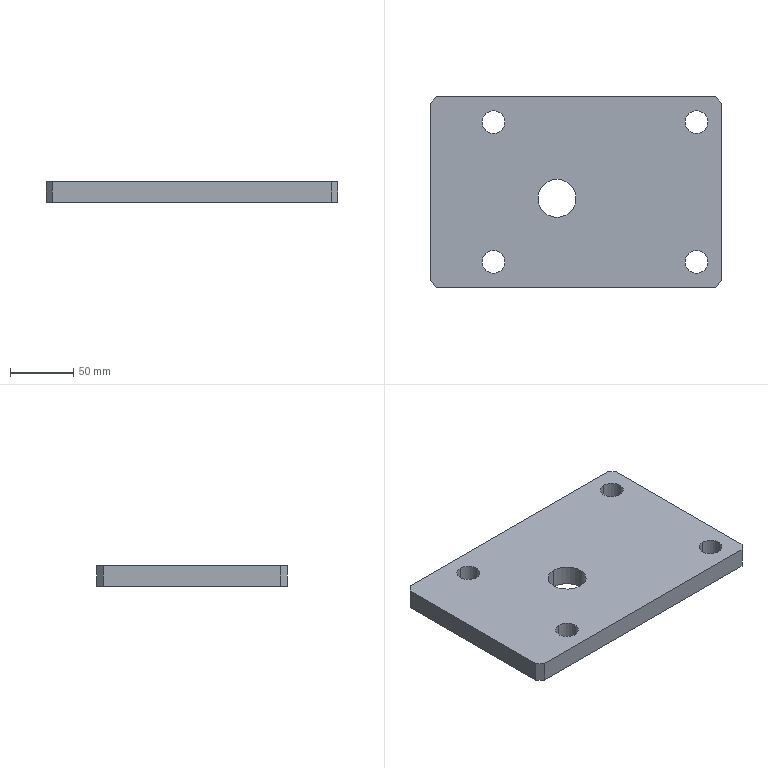Part | STEP file | [02]-1 | 1 solid | 20 faces | box 230 x 150 x 16 mm | volume 523604 mm3 | cylinder 10 | plane 10 | commonest cylinder face diameters 18 x8 30 x2